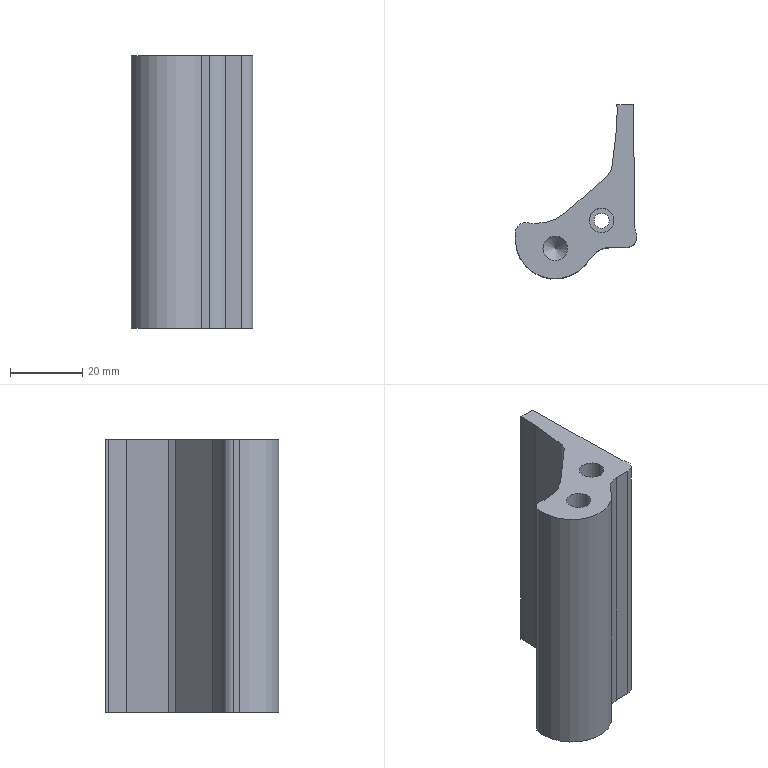Part | NX | features solid 2 | 1 solid | 28 faces | box 33.706 x 48.177 x 75.5 mm | volume 47150 mm3 | plane 16 | cylinder 10 | cone 2 | commonest cylinder face diameters 6 x4 6.8 x2 4.2 x1 5.2 x1 12 x1 22 x1
STEP:
#1=CARTESIAN_POINT('',(69.651,62.096,-5.5));
#2=VERTEX_POINT('',#1);
#3=CARTESIAN_POINT('',(69.599,62.977,-5.5));
#4=VERTEX_POINT('',#3);
#5=CARTESIAN_POINT('',(69.651,62.096,-5.5));
#6=DIRECTION('',(-0.05848,0.9983,0.));
#7=VECTOR('',#6,1000.);
#8=LINE('',#5,#7);
#9=EDGE_CURVE('',#2,#4,#8,.T.);
#10=ORIENTED_EDGE('',*,*,#9,.T.);
#11=CARTESIAN_POINT('',(74.154,62.977,-5.5));
#12=VERTEX_POINT('',#11);
#13=CARTESIAN_POINT('',(34.069,62.977,-5.5));
#14=DIRECTION('',(1.,0.,0.));
#15=VECTOR('',#14,1000.);
#16=LINE('',#13,#15);
#17=EDGE_CURVE('',#4,#12,#16,.T.);
#18=ORIENTED_EDGE('',*,*,#17,.T.);
#19=CARTESIAN_POINT('',(74.585,28.908,-5.5));
#20=VERTEX_POINT('',#19);
#21=CARTESIAN_POINT('',(73.838,88.007,-5.5));
#22=DIRECTION('',(0.01263,-0.9999,0.));
#23=VECTOR('',#22,1000.);
#24=LINE('',#21,#23);
#25=EDGE_CURVE('',#12,#20,#24,.T.);
#26=ORIENTED_EDGE('',*,*,#25,.T.);
#27=CARTESIAN_POINT('',(74.85,27.712,-5.5));
#28=VERTEX_POINT('',#27);
#29=CARTESIAN_POINT('',(77.584,28.946,-5.5));
#30=DIRECTION('',(0.,0.,1.));
#31=DIRECTION('',(1.,0.,0.));
#32=AXIS2_PLACEMENT_3D('',#29,#30,#31);
#33=CIRCLE('',#32,3.);
#34=EDGE_CURVE('',#20,#28,#33,.T.);
#35=ORIENTED_EDGE('',*,*,#34,.T.);
#36=CARTESIAN_POINT('',(72.115,23.479,-5.5));
#37=VERTEX_POINT('',#36);
#38=CARTESIAN_POINT('',(72.115,26.479,-5.5));
#39=DIRECTION('',(0.,0.,-1.));
#40=DIRECTION('',(1.,0.,0.));
#41=AXIS2_PLACEMENT_3D('',#38,#39,#40);
#42=CIRCLE('',#41,3.);
#43=EDGE_CURVE('',#28,#37,#42,.T.);
#44=ORIENTED_EDGE('',*,*,#43,.T.);
#45=CARTESIAN_POINT('',(67.618,23.479,-5.5));
#46=VERTEX_POINT('',#45);
#47=CARTESIAN_POINT('',(72.115,23.479,-5.5));
#48=DIRECTION('',(-1.,0.,0.));
#49=VECTOR('',#48,1000.);
#50=LINE('',#47,#49);
#51=EDGE_CURVE('',#37,#46,#50,.T.);
#52=ORIENTED_EDGE('',*,*,#51,.T.);
#53=CARTESIAN_POINT('',(63.022,21.335,-5.5));
#54=VERTEX_POINT('',#53);
#55=CARTESIAN_POINT('',(67.618,17.479,-5.5));
#56=DIRECTION('',(0.,0.,1.));
#57=DIRECTION('',(1.,0.,0.));
#58=AXIS2_PLACEMENT_3D('',#55,#56,#57);
#59=CIRCLE('',#58,6.);
#60=EDGE_CURVE('',#46,#54,#59,.T.);
#61=ORIENTED_EDGE('',*,*,#60,.T.);
#62=CARTESIAN_POINT('',(60.835,18.729,-5.5));
#63=VERTEX_POINT('',#62);
#64=CARTESIAN_POINT('',(63.022,21.335,-5.5));
#65=DIRECTION('',(-0.6428,-0.766,0.));
#66=VECTOR('',#65,1000.);
#67=LINE('',#64,#66);
#68=EDGE_CURVE('',#54,#63,#67,.T.);
#69=ORIENTED_EDGE('',*,*,#68,.T.);
#70=CARTESIAN_POINT('',(41.409,25.8,-5.5));
#71=VERTEX_POINT('',#70);
#72=CARTESIAN_POINT('',(52.409,25.8,-5.5));
#73=DIRECTION('',(0.,0.,-1.));
#74=DIRECTION('',(1.,0.,0.));
#75=AXIS2_PLACEMENT_3D('',#72,#73,#74);
#76=CIRCLE('',#75,11.);
#77=EDGE_CURVE('',#63,#71,#76,.T.);
#78=ORIENTED_EDGE('',*,*,#77,.T.);
#79=CARTESIAN_POINT('',(41.409,27.407,-5.5));
#80=VERTEX_POINT('',#79);
#81=CARTESIAN_POINT('',(41.409,25.8,-5.5));
#82=DIRECTION('',(0.,1.,0.));
#83=VECTOR('',#82,1000.);
#84=LINE('',#81,#83);
#85=EDGE_CURVE('',#71,#80,#84,.T.);
#86=ORIENTED_EDGE('',*,*,#85,.T.);
#87=CARTESIAN_POINT('',(45.41,30.236,-5.5));
#88=VERTEX_POINT('',#87);
#89=CARTESIAN_POINT('',(44.409,27.407,-5.5));
#90=DIRECTION('',(0.,0.,-1.));
#91=DIRECTION('',(1.,0.,0.));
#92=AXIS2_PLACEMENT_3D('',#89,#90,#91);
#93=CIRCLE('',#92,3.);
#94=EDGE_CURVE('',#80,#88,#93,.T.);
#95=ORIENTED_EDGE('',*,*,#94,.T.);
#96=CARTESIAN_POINT('',(46.789,30.088,-5.5));
#97=VERTEX_POINT('',#96);
#98=CARTESIAN_POINT('',(46.411,33.064,-5.5));
#99=DIRECTION('',(0.,0.,1.));
#100=DIRECTION('',(1.,0.,0.));
#101=AXIS2_PLACEMENT_3D('',#98,#99,#100);
#102=CIRCLE('',#101,3.);
#103=EDGE_CURVE('',#88,#97,#102,.T.);
#104=ORIENTED_EDGE('',*,*,#103,.T.);
#105=CARTESIAN_POINT('',(49.999,30.496,-5.5));
#106=VERTEX_POINT('',#105);
#107=CARTESIAN_POINT('',(46.789,30.088,-5.5));
#108=DIRECTION('',(0.992,0.1263,0.));
#109=VECTOR('',#108,1000.);
#110=LINE('',#107,#109);
#111=EDGE_CURVE('',#97,#106,#110,.T.);
#112=ORIENTED_EDGE('',*,*,#111,.T.);
#113=CARTESIAN_POINT('',(52.574,31.362,-5.5));
#114=VERTEX_POINT('',#113);
#115=CARTESIAN_POINT('',(49.999,30.496,-5.5));
#116=DIRECTION('',(0.9478,0.3189,0.));
#117=VECTOR('',#116,1000.);
#118=LINE('',#115,#117);
#119=EDGE_CURVE('',#106,#114,#118,.T.);
#120=ORIENTED_EDGE('',*,*,#119,.T.);
#121=CARTESIAN_POINT('',(55.429,33.204,-5.5));
#122=VERTEX_POINT('',#121);
#123=CARTESIAN_POINT('',(52.574,31.362,-5.5));
#124=DIRECTION('',(0.8403,0.5421,0.));
#125=VECTOR('',#124,1000.);
#126=LINE('',#123,#125);
#127=EDGE_CURVE('',#114,#122,#126,.T.);
#128=ORIENTED_EDGE('',*,*,#127,.T.);
#129=CARTESIAN_POINT('',(67.248,43.597,-5.5));
#130=VERTEX_POINT('',#129);
#131=CARTESIAN_POINT('',(55.429,33.204,-5.5));
#132=DIRECTION('',(0.7509,0.6604,0.));
#133=VECTOR('',#132,1000.);
#134=LINE('',#131,#133);
#135=EDGE_CURVE('',#122,#130,#134,.T.);
#136=ORIENTED_EDGE('',*,*,#135,.T.);
#137=CARTESIAN_POINT('',(68.162,45.368,-5.5));
#138=VERTEX_POINT('',#137);
#139=CARTESIAN_POINT('',(67.248,43.597,-5.5));
#140=DIRECTION('',(0.459,0.8885,0.));
#141=VECTOR('',#140,1000.);
#142=LINE('',#139,#141);
#143=EDGE_CURVE('',#130,#138,#142,.T.);
#144=ORIENTED_EDGE('',*,*,#143,.T.);
#145=CARTESIAN_POINT('',(69.58,57.142,-5.5));
#146=VERTEX_POINT('',#145);
#147=CARTESIAN_POINT('',(68.162,45.368,-5.5));
#148=DIRECTION('',(0.1195,0.9928,0.));
#149=VECTOR('',#148,1000.);
#150=LINE('',#147,#149);
#151=EDGE_CURVE('',#138,#146,#150,.T.);
#152=ORIENTED_EDGE('',*,*,#151,.T.);
#153=CARTESIAN_POINT('',(69.58,57.142,-5.5));
#154=DIRECTION('',(0.01432,0.9999,0.));
#155=VECTOR('',#154,1000.);
#156=LINE('',#153,#155);
#157=EDGE_CURVE('',#146,#2,#156,.T.);
#158=ORIENTED_EDGE('',*,*,#157,.T.);
#159=EDGE_LOOP('',(#10,#18,#26,#35,#44,#52,#61,#69,#78,#86,#95,#104,#112,#120,#128,#136,#144,#152,#158));
#160=FACE_BOUND('',#159,.T.);
#161=CARTESIAN_POINT('',(63.263,31.,-5.5));
#162=VERTEX_POINT('',#161);
#163=CARTESIAN_POINT('',(65.363,31.,-5.5));
#164=DIRECTION('',(0.,0.,-1.));
#165=DIRECTION('',(-1.,0.,0.));
#166=AXIS2_PLACEMENT_3D('',#163,#164,#165);
#167=CIRCLE('',#166,2.1);
#168=EDGE_CURVE('',#162,#162,#167,.T.);
#169=ORIENTED_EDGE('',*,*,#168,.F.);
#170=EDGE_LOOP('',(#169));
#171=FACE_BOUND('',#170,.T.);
#172=CARTESIAN_POINT('',(49.9,23.2,-5.5));
#173=VERTEX_POINT('',#172);
#174=CARTESIAN_POINT('',(52.5,23.2,-5.5));
#175=DIRECTION('',(0.,0.,-1.));
#176=DIRECTION('',(-1.,0.,0.));
#177=AXIS2_PLACEMENT_3D('',#174,#175,#176);
#178=CIRCLE('',#177,2.6);
#179=EDGE_CURVE('',#173,#173,#178,.F.);
#180=ORIENTED_EDGE('',*,*,#179,.T.);
#181=EDGE_LOOP('',(#180));
#182=FACE_BOUND('',#181,.T.);
#183=CARTESIAN_POINT('',(34.069,110.84,-5.5));
#184=DIRECTION('',(0.,0.,-1.));
#185=DIRECTION('',(-1.,0.,0.));
#186=AXIS2_PLACEMENT_3D('',#183,#184,#185);
#187=PLANE('',#186);
#188=ADVANCED_FACE('',(#160,#171,#182),#187,.T.);
#189=CARTESIAN_POINT('',(74.154,62.977,70.));
#190=VERTEX_POINT('',#189);
#191=CARTESIAN_POINT('',(74.585,28.908,70.));
#192=VERTEX_POINT('',#191);
#193=CARTESIAN_POINT('',(73.838,88.007,70.));
#194=DIRECTION('',(0.01263,-0.9999,0.));
#195=VECTOR('',#194,1000.);
#196=LINE('',#193,#195);
#197=EDGE_CURVE('',#190,#192,#196,.T.);
#198=ORIENTED_EDGE('',*,*,#197,.F.);
#199=CARTESIAN_POINT('',(69.599,62.977,70.));
#200=VERTEX_POINT('',#199);
#201=CARTESIAN_POINT('',(-37.5,62.977,70.));
#202=DIRECTION('',(-1.,0.,0.));
#203=VECTOR('',#202,1000.);
#204=LINE('',#201,#203);
#205=EDGE_CURVE('',#200,#190,#204,.F.);
#206=ORIENTED_EDGE('',*,*,#205,.F.);
#207=CARTESIAN_POINT('',(69.651,62.096,70.));
#208=VERTEX_POINT('',#207);
#209=CARTESIAN_POINT('',(69.651,62.096,70.));
#210=DIRECTION('',(-0.05848,0.9983,0.));
#211=VECTOR('',#210,1000.);
#212=LINE('',#209,#211);
#213=EDGE_CURVE('',#200,#208,#212,.F.);
#214=ORIENTED_EDGE('',*,*,#213,.T.);
#215=CARTESIAN_POINT('',(69.58,57.142,70.));
#216=VERTEX_POINT('',#215);
#217=CARTESIAN_POINT('',(69.58,57.142,70.));
#218=DIRECTION('',(0.01432,0.9999,0.));
#219=VECTOR('',#218,1000.);
#220=LINE('',#217,#219);
#221=EDGE_CURVE('',#208,#216,#220,.F.);
#222=ORIENTED_EDGE('',*,*,#221,.T.);
#223=CARTESIAN_POINT('',(68.162,45.368,70.));
#224=VERTEX_POINT('',#223);
#225=CARTESIAN_POINT('',(68.162,45.368,70.));
#226=DIRECTION('',(0.1195,0.9928,0.));
#227=VECTOR('',#226,1000.);
#228=LINE('',#225,#227);
#229=EDGE_CURVE('',#216,#224,#228,.F.);
#230=ORIENTED_EDGE('',*,*,#229,.T.);
#231=CARTESIAN_POINT('',(67.248,43.597,70.));
#232=VERTEX_POINT('',#231);
#233=CARTESIAN_POINT('',(67.248,43.597,70.));
#234=DIRECTION('',(0.459,0.8885,0.));
#235=VECTOR('',#234,1000.);
#236=LINE('',#233,#235);
#237=EDGE_CURVE('',#224,#232,#236,.F.);
#238=ORIENTED_EDGE('',*,*,#237,.T.);
#239=CARTESIAN_POINT('',(55.429,33.204,70.));
#240=VERTEX_POINT('',#239);
#241=CARTESIAN_POINT('',(55.429,33.204,70.));
#242=DIRECTION('',(0.7509,0.6604,0.));
#243=VECTOR('',#242,1000.);
#244=LINE('',#241,#243);
#245=EDGE_CURVE('',#232,#240,#244,.F.);
#246=ORIENTED_EDGE('',*,*,#245,.T.);
#247=CARTESIAN_POINT('',(52.574,31.362,70.));
#248=VERTEX_POINT('',#247);
#249=CARTESIAN_POINT('',(52.574,31.362,70.));
#250=DIRECTION('',(0.8403,0.5421,0.));
#251=VECTOR('',#250,1000.);
#252=LINE('',#249,#251);
#253=EDGE_CURVE('',#240,#248,#252,.F.);
#254=ORIENTED_EDGE('',*,*,#253,.T.);
#255=CARTESIAN_POINT('',(49.999,30.496,70.));
#256=VERTEX_POINT('',#255);
#257=CARTESIAN_POINT('',(49.999,30.496,70.));
#258=DIRECTION('',(0.9478,0.3189,0.));
#259=VECTOR('',#258,1000.);
#260=LINE('',#257,#259);
#261=EDGE_CURVE('',#248,#256,#260,.F.);
#262=ORIENTED_EDGE('',*,*,#261,.T.);
#263=CARTESIAN_POINT('',(46.789,30.088,70.));
#264=VERTEX_POINT('',#263);
#265=CARTESIAN_POINT('',(46.789,30.088,70.));
#266=DIRECTION('',(0.992,0.1263,0.));
#267=VECTOR('',#266,1000.);
#268=LINE('',#265,#267);
#269=EDGE_CURVE('',#256,#264,#268,.F.);
#270=ORIENTED_EDGE('',*,*,#269,.T.);
#271=CARTESIAN_POINT('',(45.41,30.236,70.));
#272=VERTEX_POINT('',#271);
#273=CARTESIAN_POINT('',(46.411,33.064,70.));
#274=DIRECTION('',(0.,0.,1.));
#275=DIRECTION('',(1.,0.,0.));
#276=AXIS2_PLACEMENT_3D('',#273,#274,#275);
#277=CIRCLE('',#276,3.);
#278=EDGE_CURVE('',#272,#264,#277,.T.);
#279=ORIENTED_EDGE('',*,*,#278,.F.);
#280=CARTESIAN_POINT('',(41.409,27.407,70.));
#281=VERTEX_POINT('',#280);
#282=CARTESIAN_POINT('',(44.409,27.407,70.));
#283=DIRECTION('',(0.,0.,1.));
#284=DIRECTION('',(1.,0.,0.));
#285=AXIS2_PLACEMENT_3D('',#282,#283,#284);
#286=CIRCLE('',#285,3.);
#287=EDGE_CURVE('',#281,#272,#286,.F.);
#288=ORIENTED_EDGE('',*,*,#287,.F.);
#289=CARTESIAN_POINT('',(41.409,25.8,70.));
#290=VERTEX_POINT('',#289);
#291=CARTESIAN_POINT('',(41.409,25.8,70.));
#292=DIRECTION('',(0.,1.,0.));
#293=VECTOR('',#292,1000.);
#294=LINE('',#291,#293);
#295=EDGE_CURVE('',#290,#281,#294,.T.);
#296=ORIENTED_EDGE('',*,*,#295,.F.);
#297=CARTESIAN_POINT('',(60.835,18.729,70.));
#298=VERTEX_POINT('',#297);
#299=CARTESIAN_POINT('',(52.409,25.8,70.));
#300=DIRECTION('',(0.,0.,1.));
#301=DIRECTION('',(1.,0.,0.));
#302=AXIS2_PLACEMENT_3D('',#299,#300,#301);
#303=CIRCLE('',#302,11.);
#304=EDGE_CURVE('',#298,#290,#303,.F.);
#305=ORIENTED_EDGE('',*,*,#304,.F.);
#306=CARTESIAN_POINT('',(63.022,21.335,70.));
#307=VERTEX_POINT('',#306);
#308=CARTESIAN_POINT('',(63.022,21.335,70.));
#309=DIRECTION('',(-0.6428,-0.766,0.));
#310=VECTOR('',#309,1000.);
#311=LINE('',#308,#310);
#312=EDGE_CURVE('',#307,#298,#311,.T.);
#313=ORIENTED_EDGE('',*,*,#312,.F.);
#314=CARTESIAN_POINT('',(67.618,23.479,70.));
#315=VERTEX_POINT('',#314);
#316=CARTESIAN_POINT('',(67.618,17.479,70.));
#317=DIRECTION('',(0.,0.,1.));
#318=DIRECTION('',(1.,0.,0.));
#319=AXIS2_PLACEMENT_3D('',#316,#317,#318);
#320=CIRCLE('',#319,6.);
#321=EDGE_CURVE('',#315,#307,#320,.T.);
#322=ORIENTED_EDGE('',*,*,#321,.F.);
#323=CARTESIAN_POINT('',(72.115,23.479,70.));
#324=VERTEX_POINT('',#323);
#325=CARTESIAN_POINT('',(72.115,23.479,70.));
#326=DIRECTION('',(-1.,0.,0.));
#327=VECTOR('',#326,1000.);
#328=LINE('',#325,#327);
#329=EDGE_CURVE('',#324,#315,#328,.T.);
#330=ORIENTED_EDGE('',*,*,#329,.F.);
#331=CARTESIAN_POINT('',(74.85,27.712,70.));
#332=VERTEX_POINT('',#331);
#333=CARTESIAN_POINT('',(72.115,26.479,70.));
#334=DIRECTION('',(0.,0.,1.));
#335=DIRECTION('',(1.,0.,0.));
#336=AXIS2_PLACEMENT_3D('',#333,#334,#335);
#337=CIRCLE('',#336,3.);
#338=EDGE_CURVE('',#332,#324,#337,.F.);
#339=ORIENTED_EDGE('',*,*,#338,.F.);
#340=CARTESIAN_POINT('',(77.584,28.946,70.));
#341=DIRECTION('',(0.,0.,1.));
#342=DIRECTION('',(1.,0.,0.));
#343=AXIS2_PLACEMENT_3D('',#340,#341,#342);
#344=CIRCLE('',#343,3.);
#345=EDGE_CURVE('',#192,#332,#344,.T.);
#346=ORIENTED_EDGE('',*,*,#345,.F.);
#347=EDGE_LOOP('',(#198,#206,#214,#222,#230,#238,#246,#254,#262,#270,#279,#288,#296,#305,#313,#322,#330,#339,#346));
#348=FACE_BOUND('',#347,.T.);
#349=CARTESIAN_POINT('',(68.763,31.,70.));
#350=VERTEX_POINT('',#349);
#351=CARTESIAN_POINT('',(65.363,31.,70.));
#352=DIRECTION('',(0.,0.,1.));
#353=DIRECTION('',(1.,0.,0.));
#354=AXIS2_PLACEMENT_3D('',#351,#352,#353);
#355=CIRCLE('',#354,3.4);
#356=EDGE_CURVE('',#350,#350,#355,.T.);
#357=ORIENTED_EDGE('',*,*,#356,.F.);
#358=EDGE_LOOP('',(#357));
#359=FACE_BOUND('',#358,.T.);
#360=CARTESIAN_POINT('',(55.9,23.2,70.));
#361=VERTEX_POINT('',#360);
#362=CARTESIAN_POINT('',(52.5,23.2,70.));
#363=DIRECTION('',(0.,0.,-1.));
#364=DIRECTION('',(1.,0.,0.));
#365=AXIS2_PLACEMENT_3D('',#362,#363,#364);
#366=CIRCLE('',#365,3.4);
#367=EDGE_CURVE('',#361,#361,#366,.T.);
#368=ORIENTED_EDGE('',*,*,#367,.T.);
#369=EDGE_LOOP('',(#368));
#370=FACE_BOUND('',#369,.T.);
#371=CARTESIAN_POINT('',(-37.5,0.,70.));
#372=DIRECTION('',(0.,0.,1.));
#373=DIRECTION('',(1.,0.,0.));
#374=AXIS2_PLACEMENT_3D('',#371,#372,#373);
#375=PLANE('',#374);
#376=ADVANCED_FACE('',(#348,#359,#370),#375,.T.);
#377=ORIENTED_EDGE('',*,*,#17,.F.);
#378=CARTESIAN_POINT('',(69.599,62.977,40.));
#379=DIRECTION('',(0.,0.,-1.));
#380=VECTOR('',#379,1000.);
#381=LINE('',#378,#380);
#382=EDGE_CURVE('',#200,#4,#381,.T.);
#383=ORIENTED_EDGE('',*,*,#382,.F.);
#384=ORIENTED_EDGE('',*,*,#205,.T.);
#385=CARTESIAN_POINT('',(74.154,62.977,40.));
#386=DIRECTION('',(0.,0.,1.));
#387=VECTOR('',#386,1000.);
#388=LINE('',#385,#387);
#389=EDGE_CURVE('',#190,#12,#388,.F.);
#390=ORIENTED_EDGE('',*,*,#389,.T.);
#391=EDGE_LOOP('',(#377,#383,#384,#390));
#392=FACE_BOUND('',#391,.T.);
#393=CARTESIAN_POINT('',(7.645,62.977,0.));
#394=DIRECTION('',(0.,1.,0.));
#395=DIRECTION('',(0.,0.,1.));
#396=AXIS2_PLACEMENT_3D('',#393,#394,#395);
#397=PLANE('',#396);
#398=ADVANCED_FACE('',(#392),#397,.T.);
#399=CARTESIAN_POINT('',(63.263,31.,29.5));
#400=VERTEX_POINT('',#399);
#401=CARTESIAN_POINT('',(65.363,31.,29.5));
#402=DIRECTION('',(0.,0.,-1.));
#403=DIRECTION('',(-1.,0.,0.));
#404=AXIS2_PLACEMENT_3D('',#401,#402,#403);
#405=CIRCLE('',#404,2.1);
#406=EDGE_CURVE('',#400,#400,#405,.T.);
#407=ORIENTED_EDGE('',*,*,#406,.T.);
#408=EDGE_LOOP('',(#407));
#409=FACE_BOUND('',#408,.T.);
#410=CARTESIAN_POINT('',(68.763,31.,29.5));
#411=VERTEX_POINT('',#410);
#412=CARTESIAN_POINT('',(65.363,31.,29.5));
#413=DIRECTION('',(0.,0.,1.));
#414=DIRECTION('',(1.,0.,0.));
#415=AXIS2_PLACEMENT_3D('',#412,#413,#414);
#416=CIRCLE('',#415,3.4);
#417=EDGE_CURVE('',#411,#411,#416,.F.);
#418=ORIENTED_EDGE('',*,*,#417,.F.);
#419=EDGE_LOOP('',(#418));
#420=FACE_BOUND('',#419,.T.);
#421=CARTESIAN_POINT('',(65.363,31.,29.5));
#422=DIRECTION('',(0.,0.,-1.));
#423=DIRECTION('',(-1.,0.,0.));
#424=AXIS2_PLACEMENT_3D('',#421,#422,#423);
#425=PLANE('',#424);
#426=ADVANCED_FACE('',(#409,#420),#425,.F.);
#427=ORIENTED_EDGE('',*,*,#168,.T.);
#428=EDGE_LOOP('',(#427));
#429=FACE_BOUND('',#428,.T.);
#430=ORIENTED_EDGE('',*,*,#406,.F.);
#431=EDGE_LOOP('',(#430));
#432=FACE_BOUND('',#431,.T.);
#433=CARTESIAN_POINT('',(65.363,31.,32.5));
#434=DIRECTION('',(0.,0.,-1.));
#435=DIRECTION('',(1.,0.,0.));
#436=AXIS2_PLACEMENT_3D('',#433,#434,#435);
#437=CYLINDRICAL_SURFACE('',#436,2.1);
#438=ADVANCED_FACE('',(#429,#432),#437,.F.);
#439=CARTESIAN_POINT('',(74.585,28.908,40.));
#440=DIRECTION('',(0.,0.,-1.));
#441=VECTOR('',#440,1000.);
#442=LINE('',#439,#441);
#443=EDGE_CURVE('',#192,#20,#442,.T.);
#444=ORIENTED_EDGE('',*,*,#443,.F.);
#445=ORIENTED_EDGE('',*,*,#345,.T.);
#446=CARTESIAN_POINT('',(74.85,27.712,40.));
#447=DIRECTION('',(0.,0.,-1.));
#448=VECTOR('',#447,1000.);
#449=LINE('',#446,#448);
#450=EDGE_CURVE('',#332,#28,#449,.T.);
#451=ORIENTED_EDGE('',*,*,#450,.T.);
#452=ORIENTED_EDGE('',*,*,#34,.F.);
#453=EDGE_LOOP('',(#444,#445,#451,#452));
#454=FACE_BOUND('',#453,.T.);
#455=CARTESIAN_POINT('',(77.584,28.946,40.));
#456=DIRECTION('',(0.,0.,-1.));
#457=DIRECTION('',(-1.,0.,0.));
#458=AXIS2_PLACEMENT_3D('',#455,#456,#457);
#459=CYLINDRICAL_SURFACE('',#458,3.);
#460=ADVANCED_FACE('',(#454),#459,.F.);
#461=ORIENTED_EDGE('',*,*,#450,.F.);
#462=ORIENTED_EDGE('',*,*,#338,.T.);
#463=CARTESIAN_POINT('',(72.115,23.479,40.));
#464=DIRECTION('',(0.,0.,-1.));
#465=VECTOR('',#464,1000.);
#466=LINE('',#463,#465);
#467=EDGE_CURVE('',#324,#37,#466,.T.);
#468=ORIENTED_EDGE('',*,*,#467,.T.);
#469=ORIENTED_EDGE('',*,*,#43,.F.);
#470=EDGE_LOOP('',(#461,#462,#468,#469));
#471=FACE_BOUND('',#470,.T.);
#472=CARTESIAN_POINT('',(72.115,26.479,40.));
#473=DIRECTION('',(0.,0.,-1.));
#474=DIRECTION('',(-1.,0.,0.));
#475=AXIS2_PLACEMENT_3D('',#472,#473,#474);
#476=CYLINDRICAL_SURFACE('',#475,3.);
#477=ADVANCED_FACE('',(#471),#476,.T.);
#478=ORIENTED_EDGE('',*,*,#467,.F.);
#479=ORIENTED_EDGE('',*,*,#329,.T.);
#480=CARTESIAN_POINT('',(67.618,23.479,40.));
#481=DIRECTION('',(0.,0.,-1.));
#482=VECTOR('',#481,1000.);
#483=LINE('',#480,#482);
#484=EDGE_CURVE('',#315,#46,#483,.T.);
#485=ORIENTED_EDGE('',*,*,#484,.T.);
#486=ORIENTED_EDGE('',*,*,#51,.F.);
#487=EDGE_LOOP('',(#478,#479,#485,#486));
#488=FACE_BOUND('',#487,.T.);
#489=CARTESIAN_POINT('',(72.115,23.479,40.));
#490=DIRECTION('',(0.,-1.,0.));
#491=DIRECTION('',(1.,0.,0.));
#492=AXIS2_PLACEMENT_3D('',#489,#490,#491);
#493=PLANE('',#492);
#494=ADVANCED_FACE('',(#488),#493,.T.);
#495=ORIENTED_EDGE('',*,*,#484,.F.);
#496=ORIENTED_EDGE('',*,*,#321,.T.);
#497=CARTESIAN_POINT('',(63.022,21.335,40.));
#498=DIRECTION('',(0.,0.,-1.));
#499=VECTOR('',#498,1000.);
#500=LINE('',#497,#499);
#501=EDGE_CURVE('',#307,#54,#500,.T.);
#502=ORIENTED_EDGE('',*,*,#501,.T.);
#503=ORIENTED_EDGE('',*,*,#60,.F.);
#504=EDGE_LOOP('',(#495,#496,#502,#503));
#505=FACE_BOUND('',#504,.T.);
#506=CARTESIAN_POINT('',(67.618,17.479,40.));
#507=DIRECTION('',(0.,0.,-1.));
#508=DIRECTION('',(-1.,0.,0.));
#509=AXIS2_PLACEMENT_3D('',#506,#507,#508);
#510=CYLINDRICAL_SURFACE('',#509,6.);
#511=ADVANCED_FACE('',(#505),#510,.F.);
#512=ORIENTED_EDGE('',*,*,#501,.F.);
#513=ORIENTED_EDGE('',*,*,#312,.T.);
#514=CARTESIAN_POINT('',(60.835,18.729,40.));
#515=DIRECTION('',(0.,0.,-1.));
#516=VECTOR('',#515,1000.);
#517=LINE('',#514,#516);
#518=EDGE_CURVE('',#298,#63,#517,.T.);
#519=ORIENTED_EDGE('',*,*,#518,.T.);
#520=ORIENTED_EDGE('',*,*,#68,.F.);
#521=EDGE_LOOP('',(#512,#513,#519,#520));
#522=FACE_BOUND('',#521,.T.);
#523=CARTESIAN_POINT('',(63.022,21.335,40.));
#524=DIRECTION('',(0.766,-0.6428,0.));
#525=DIRECTION('',(0.6428,0.766,0.));
#526=AXIS2_PLACEMENT_3D('',#523,#524,#525);
#527=PLANE('',#526);
#528=ADVANCED_FACE('',(#522),#527,.T.);
#529=ORIENTED_EDGE('',*,*,#518,.F.);
#530=ORIENTED_EDGE('',*,*,#304,.T.);
#531=CARTESIAN_POINT('',(41.409,25.8,40.));
#532=DIRECTION('',(0.,0.,-1.));
#533=VECTOR('',#532,1000.);
#534=LINE('',#531,#533);
#535=EDGE_CURVE('',#290,#71,#534,.T.);
#536=ORIENTED_EDGE('',*,*,#535,.T.);
#537=ORIENTED_EDGE('',*,*,#77,.F.);
#538=EDGE_LOOP('',(#529,#530,#536,#537));
#539=FACE_BOUND('',#538,.T.);
#540=CARTESIAN_POINT('',(52.409,25.8,40.));
#541=DIRECTION('',(0.,0.,-1.));
#542=DIRECTION('',(-1.,0.,0.));
#543=AXIS2_PLACEMENT_3D('',#540,#541,#542);
#544=CYLINDRICAL_SURFACE('',#543,11.);
#545=ADVANCED_FACE('',(#539),#544,.T.);
#546=ORIENTED_EDGE('',*,*,#535,.F.);
#547=ORIENTED_EDGE('',*,*,#295,.T.);
#548=CARTESIAN_POINT('',(41.409,27.407,40.));
#549=DIRECTION('',(0.,0.,-1.));
#550=VECTOR('',#549,1000.);
#551=LINE('',#548,#550);
#552=EDGE_CURVE('',#281,#80,#551,.T.);
#553=ORIENTED_EDGE('',*,*,#552,.T.);
#554=ORIENTED_EDGE('',*,*,#85,.F.);
#555=EDGE_LOOP('',(#546,#547,#553,#554));
#556=FACE_BOUND('',#555,.T.);
#557=CARTESIAN_POINT('',(41.409,25.8,40.));
#558=DIRECTION('',(-1.,0.,0.));
#559=DIRECTION('',(0.,-1.,0.));
#560=AXIS2_PLACEMENT_3D('',#557,#558,#559);
#561=PLANE('',#560);
#562=ADVANCED_FACE('',(#556),#561,.T.);
#563=ORIENTED_EDGE('',*,*,#552,.F.);
#564=ORIENTED_EDGE('',*,*,#287,.T.);
#565=CARTESIAN_POINT('',(45.41,30.236,40.));
#566=DIRECTION('',(0.,0.,-1.));
#567=VECTOR('',#566,1000.);
#568=LINE('',#565,#567);
#569=EDGE_CURVE('',#272,#88,#568,.T.);
#570=ORIENTED_EDGE('',*,*,#569,.T.);
#571=ORIENTED_EDGE('',*,*,#94,.F.);
#572=EDGE_LOOP('',(#563,#564,#570,#571));
#573=FACE_BOUND('',#572,.T.);
#574=CARTESIAN_POINT('',(44.409,27.407,40.));
#575=DIRECTION('',(0.,0.,-1.));
#576=DIRECTION('',(-1.,0.,0.));
#577=AXIS2_PLACEMENT_3D('',#574,#575,#576);
#578=CYLINDRICAL_SURFACE('',#577,3.);
#579=ADVANCED_FACE('',(#573),#578,.T.);
#580=ORIENTED_EDGE('',*,*,#278,.T.);
#581=CARTESIAN_POINT('',(46.789,30.088,40.));
#582=DIRECTION('',(0.,0.,-1.));
#583=VECTOR('',#582,1000.);
#584=LINE('',#581,#583);
#585=EDGE_CURVE('',#264,#97,#584,.T.);
#586=ORIENTED_EDGE('',*,*,#585,.T.);
#587=ORIENTED_EDGE('',*,*,#103,.F.);
#588=ORIENTED_EDGE('',*,*,#569,.F.);
#589=EDGE_LOOP('',(#580,#586,#587,#588));
#590=FACE_BOUND('',#589,.T.);
#591=CARTESIAN_POINT('',(46.411,33.064,40.));
#592=DIRECTION('',(0.,0.,-1.));
#593=DIRECTION('',(-1.,0.,0.));
#594=AXIS2_PLACEMENT_3D('',#591,#592,#593);
#595=CYLINDRICAL_SURFACE('',#594,3.);
#596=ADVANCED_FACE('',(#590),#595,.F.);
#597=ORIENTED_EDGE('',*,*,#585,.F.);
#598=ORIENTED_EDGE('',*,*,#269,.F.);
#599=CARTESIAN_POINT('',(49.999,30.496,40.));
#600=DIRECTION('',(0.,0.,-1.));
#601=VECTOR('',#600,1000.);
#602=LINE('',#599,#601);
#603=EDGE_CURVE('',#256,#106,#602,.T.);
#604=ORIENTED_EDGE('',*,*,#603,.T.);
#605=ORIENTED_EDGE('',*,*,#111,.F.);
#606=EDGE_LOOP('',(#597,#598,#604,#605));
#607=FACE_BOUND('',#606,.T.);
#608=CARTESIAN_POINT('',(46.789,30.088,40.));
#609=DIRECTION('',(-0.1263,0.992,0.));
#610=DIRECTION('',(-0.992,-0.1263,0.));
#611=AXIS2_PLACEMENT_3D('',#608,#609,#610);
#612=PLANE('',#611);
#613=ADVANCED_FACE('',(#607),#612,.T.);
#614=ORIENTED_EDGE('',*,*,#261,.F.);
#615=CARTESIAN_POINT('',(52.574,31.362,40.));
#616=DIRECTION('',(0.,0.,-1.));
#617=VECTOR('',#616,1000.);
#618=LINE('',#615,#617);
#619=EDGE_CURVE('',#248,#114,#618,.T.);
#620=ORIENTED_EDGE('',*,*,#619,.T.);
#621=ORIENTED_EDGE('',*,*,#119,.F.);
#622=ORIENTED_EDGE('',*,*,#603,.F.);
#623=EDGE_LOOP('',(#614,#620,#621,#622));
#624=FACE_BOUND('',#623,.T.);
#625=CARTESIAN_POINT('',(49.999,30.496,40.));
#626=DIRECTION('',(-0.3189,0.9478,0.));
#627=DIRECTION('',(-0.9478,-0.3189,0.));
#628=AXIS2_PLACEMENT_3D('',#625,#626,#627);
#629=PLANE('',#628);
#630=ADVANCED_FACE('',(#624),#629,.T.);
#631=ORIENTED_EDGE('',*,*,#253,.F.);
#632=CARTESIAN_POINT('',(55.429,33.204,40.));
#633=DIRECTION('',(0.,0.,-1.));
#634=VECTOR('',#633,1000.);
#635=LINE('',#632,#634);
#636=EDGE_CURVE('',#240,#122,#635,.T.);
#637=ORIENTED_EDGE('',*,*,#636,.T.);
#638=ORIENTED_EDGE('',*,*,#127,.F.);
#639=ORIENTED_EDGE('',*,*,#619,.F.);
#640=EDGE_LOOP('',(#631,#637,#638,#639));
#641=FACE_BOUND('',#640,.T.);
#642=CARTESIAN_POINT('',(52.574,31.362,40.));
#643=DIRECTION('',(-0.5421,0.8403,0.));
#644=DIRECTION('',(-0.8403,-0.5421,0.));
#645=AXIS2_PLACEMENT_3D('',#642,#643,#644);
#646=PLANE('',#645);
#647=ADVANCED_FACE('',(#641),#646,.T.);
#648=ORIENTED_EDGE('',*,*,#245,.F.);
#649=CARTESIAN_POINT('',(67.248,43.597,40.));
#650=DIRECTION('',(0.,0.,-1.));
#651=VECTOR('',#650,1000.);
#652=LINE('',#649,#651);
#653=EDGE_CURVE('',#232,#130,#652,.T.);
#654=ORIENTED_EDGE('',*,*,#653,.T.);
#655=ORIENTED_EDGE('',*,*,#135,.F.);
#656=ORIENTED_EDGE('',*,*,#636,.F.);
#657=EDGE_LOOP('',(#648,#654,#655,#656));
#658=FACE_BOUND('',#657,.T.);
#659=CARTESIAN_POINT('',(55.429,33.204,40.));
#660=DIRECTION('',(-0.6604,0.7509,0.));
#661=DIRECTION('',(-0.7509,-0.6604,0.));
#662=AXIS2_PLACEMENT_3D('',#659,#660,#661);
#663=PLANE('',#662);
#664=ADVANCED_FACE('',(#658),#663,.T.);
#665=ORIENTED_EDGE('',*,*,#237,.F.);
#666=CARTESIAN_POINT('',(68.162,45.368,40.));
#667=DIRECTION('',(0.,0.,-1.));
#668=VECTOR('',#667,1000.);
#669=LINE('',#666,#668);
#670=EDGE_CURVE('',#224,#138,#669,.T.);
#671=ORIENTED_EDGE('',*,*,#670,.T.);
#672=ORIENTED_EDGE('',*,*,#143,.F.);
#673=ORIENTED_EDGE('',*,*,#653,.F.);
#674=EDGE_LOOP('',(#665,#671,#672,#673));
#675=FACE_BOUND('',#674,.T.);
#676=CARTESIAN_POINT('',(67.248,43.597,40.));
#677=DIRECTION('',(-0.8885,0.459,0.));
#678=DIRECTION('',(-0.459,-0.8885,0.));
#679=AXIS2_PLACEMENT_3D('',#676,#677,#678);
#680=PLANE('',#679);
#681=ADVANCED_FACE('',(#675),#680,.T.);
#682=ORIENTED_EDGE('',*,*,#229,.F.);
#683=CARTESIAN_POINT('',(69.58,57.142,40.));
#684=DIRECTION('',(0.,0.,-1.));
#685=VECTOR('',#684,1000.);
#686=LINE('',#683,#685);
#687=EDGE_CURVE('',#216,#146,#686,.T.);
#688=ORIENTED_EDGE('',*,*,#687,.T.);
#689=ORIENTED_EDGE('',*,*,#151,.F.);
#690=ORIENTED_EDGE('',*,*,#670,.F.);
#691=EDGE_LOOP('',(#682,#688,#689,#690));
#692=FACE_BOUND('',#691,.T.);
#693=CARTESIAN_POINT('',(68.162,45.368,40.));
#694=DIRECTION('',(-0.9928,0.1195,0.));
#695=DIRECTION('',(-0.1195,-0.9928,0.));
#696=AXIS2_PLACEMENT_3D('',#693,#694,#695);
#697=PLANE('',#696);
#698=ADVANCED_FACE('',(#692),#697,.T.);
#699=ORIENTED_EDGE('',*,*,#221,.F.);
#700=CARTESIAN_POINT('',(69.651,62.096,40.));
#701=DIRECTION('',(0.,0.,-1.));
#702=VECTOR('',#701,1000.);
#703=LINE('',#700,#702);
#704=EDGE_CURVE('',#208,#2,#703,.T.);
#705=ORIENTED_EDGE('',*,*,#704,.T.);
#706=ORIENTED_EDGE('',*,*,#157,.F.);
#707=ORIENTED_EDGE('',*,*,#687,.F.);
#708=EDGE_LOOP('',(#699,#705,#706,#707));
#709=FACE_BOUND('',#708,.T.);
#710=CARTESIAN_POINT('',(69.58,57.142,40.));
#711=DIRECTION('',(-0.9999,0.01432,0.));
#712=DIRECTION('',(-0.01432,-0.9999,0.));
#713=AXIS2_PLACEMENT_3D('',#710,#711,#712);
#714=PLANE('',#713);
#715=ADVANCED_FACE('',(#709),#714,.T.);
#716=ORIENTED_EDGE('',*,*,#356,.T.);
#717=EDGE_LOOP('',(#716));
#718=FACE_BOUND('',#717,.T.);
#719=ORIENTED_EDGE('',*,*,#417,.T.);
#720=EDGE_LOOP('',(#719));
#721=FACE_BOUND('',#720,.T.);
#722=CARTESIAN_POINT('',(65.363,31.,29.5));
#723=DIRECTION('',(0.,0.,1.));
#724=DIRECTION('',(1.,0.,0.));
#725=AXIS2_PLACEMENT_3D('',#722,#723,#724);
#726=CYLINDRICAL_SURFACE('',#725,3.4);
#727=ADVANCED_FACE('',(#718,#721),#726,.F.);
#728=ORIENTED_EDGE('',*,*,#25,.F.);
#729=ORIENTED_EDGE('',*,*,#389,.F.);
#730=ORIENTED_EDGE('',*,*,#197,.T.);
#731=ORIENTED_EDGE('',*,*,#443,.T.);
#732=EDGE_LOOP('',(#728,#729,#730,#731));
#733=FACE_BOUND('',#732,.T.);
#734=CARTESIAN_POINT('',(73.838,88.007,40.));
#735=DIRECTION('',(0.9999,0.01263,0.));
#736=DIRECTION('',(-0.01263,0.9999,0.));
#737=AXIS2_PLACEMENT_3D('',#734,#735,#736);
#738=PLANE('',#737);
#739=ADVANCED_FACE('',(#733),#738,.T.);
#740=ORIENTED_EDGE('',*,*,#213,.F.);
#741=ORIENTED_EDGE('',*,*,#382,.T.);
#742=ORIENTED_EDGE('',*,*,#9,.F.);
#743=ORIENTED_EDGE('',*,*,#704,.F.);
#744=EDGE_LOOP('',(#740,#741,#742,#743));
#745=FACE_BOUND('',#744,.T.);
#746=CARTESIAN_POINT('',(69.651,62.096,40.));
#747=DIRECTION('',(-0.9983,-0.05848,0.));
#748=DIRECTION('',(0.05848,-0.9983,0.));
#749=AXIS2_PLACEMENT_3D('',#746,#747,#748);
#750=PLANE('',#749);
#751=ADVANCED_FACE('',(#745),#750,.T.);
#752=CARTESIAN_POINT('',(49.1,23.2,44.4));
#753=VERTEX_POINT('',#752);
#754=CARTESIAN_POINT('',(52.5,23.2,44.4));
#755=DIRECTION('',(0.,0.,-1.));
#756=DIRECTION('',(-1.,0.,0.));
#757=AXIS2_PLACEMENT_3D('',#754,#755,#756);
#758=CIRCLE('',#757,3.4);
#759=EDGE_CURVE('',#753,#753,#758,.T.);
#760=ORIENTED_EDGE('',*,*,#759,.T.);
#761=EDGE_LOOP('',(#760));
#762=FACE_BOUND('',#761,.T.);
#763=ORIENTED_EDGE('',*,*,#367,.F.);
#764=EDGE_LOOP('',(#763));
#765=FACE_BOUND('',#764,.T.);
#766=CARTESIAN_POINT('',(52.5,23.2,70.));
#767=DIRECTION('',(0.,0.,-1.));
#768=DIRECTION('',(1.,0.,0.));
#769=AXIS2_PLACEMENT_3D('',#766,#767,#768);
#770=CYLINDRICAL_SURFACE('',#769,3.4);
#771=ADVANCED_FACE('',(#762,#765),#770,.F.);
#772=CARTESIAN_POINT('',(52.5,23.2,41.));
#773=VERTEX_POINT('',#772);
#774=VERTEX_LOOP('',#773);
#775=FACE_BOUND('',#774,.T.);
#776=ORIENTED_EDGE('',*,*,#759,.F.);
#777=EDGE_LOOP('',(#776));
#778=FACE_BOUND('',#777,.T.);
#779=CARTESIAN_POINT('',(52.5,23.2,44.4));
#780=DIRECTION('',(0.,0.,1.));
#781=DIRECTION('',(1.,0.,0.));
#782=AXIS2_PLACEMENT_3D('',#779,#780,#781);
#783=CONICAL_SURFACE('',#782,3.4,0.7854);
#784=ADVANCED_FACE('',(#775,#778),#783,.F.);
#785=CARTESIAN_POINT('',(49.9,23.2,15.9));
#786=VERTEX_POINT('',#785);
#787=CARTESIAN_POINT('',(52.5,23.2,15.9));
#788=DIRECTION('',(0.,0.,-1.));
#789=DIRECTION('',(-1.,0.,0.));
#790=AXIS2_PLACEMENT_3D('',#787,#788,#789);
#791=CIRCLE('',#790,2.6);
#792=EDGE_CURVE('',#786,#786,#791,.F.);
#793=ORIENTED_EDGE('',*,*,#792,.T.);
#794=EDGE_LOOP('',(#793));
#795=FACE_BOUND('',#794,.T.);
#796=ORIENTED_EDGE('',*,*,#179,.F.);
#797=EDGE_LOOP('',(#796));
#798=FACE_BOUND('',#797,.T.);
#799=CARTESIAN_POINT('',(52.5,23.2,-5.5));
#800=DIRECTION('',(0.,0.,1.));
#801=DIRECTION('',(1.,0.,0.));
#802=AXIS2_PLACEMENT_3D('',#799,#800,#801);
#803=CYLINDRICAL_SURFACE('',#802,2.6);
#804=ADVANCED_FACE('',(#795,#798),#803,.F.);
#805=CARTESIAN_POINT('',(52.5,23.2,18.5));
#806=VERTEX_POINT('',#805);
#807=VERTEX_LOOP('',#806);
#808=FACE_BOUND('',#807,.T.);
#809=ORIENTED_EDGE('',*,*,#792,.F.);
#810=EDGE_LOOP('',(#809));
#811=FACE_BOUND('',#810,.T.);
#812=CARTESIAN_POINT('',(52.5,23.2,15.9));
#813=DIRECTION('',(0.,0.,-1.));
#814=DIRECTION('',(-1.,0.,0.));
#815=AXIS2_PLACEMENT_3D('',#812,#813,#814);
#816=CONICAL_SURFACE('',#815,2.599,0.7854);
#817=ADVANCED_FACE('',(#808,#811),#816,.F.);
#818=CLOSED_SHELL('',(#188,#376,#398,#426,#438,#460,#477,#494,#511,#528,#545,#562,#579,#596,#613,#630,#647,#664,#681,#698,#715,#727,#739,#751,#771,#784,#804,#817));
#819=MANIFOLD_SOLID_BREP('',#818);
#820=(LENGTH_UNIT()NAMED_UNIT(*)SI_UNIT(.MILLI.,.METRE.));
#821=UNCERTAINTY_MEASURE_WITH_UNIT(LENGTH_MEASURE(0.00001),#820,'','');
#822=(NAMED_UNIT(*)PLANE_ANGLE_UNIT()SI_UNIT($,.RADIAN.));
#823=(NAMED_UNIT(*)SI_UNIT($,.STERADIAN.)SOLID_ANGLE_UNIT());
#824=(GEOMETRIC_REPRESENTATION_CONTEXT(3)GLOBAL_UNCERTAINTY_ASSIGNED_CONTEXT((#821))GLOBAL_UNIT_ASSIGNED_CONTEXT((#820,#822,#823))REPRESENTATION_CONTEXT('',''));
#825=ADVANCED_BREP_SHAPE_REPRESENTATION('',(#819),#824);